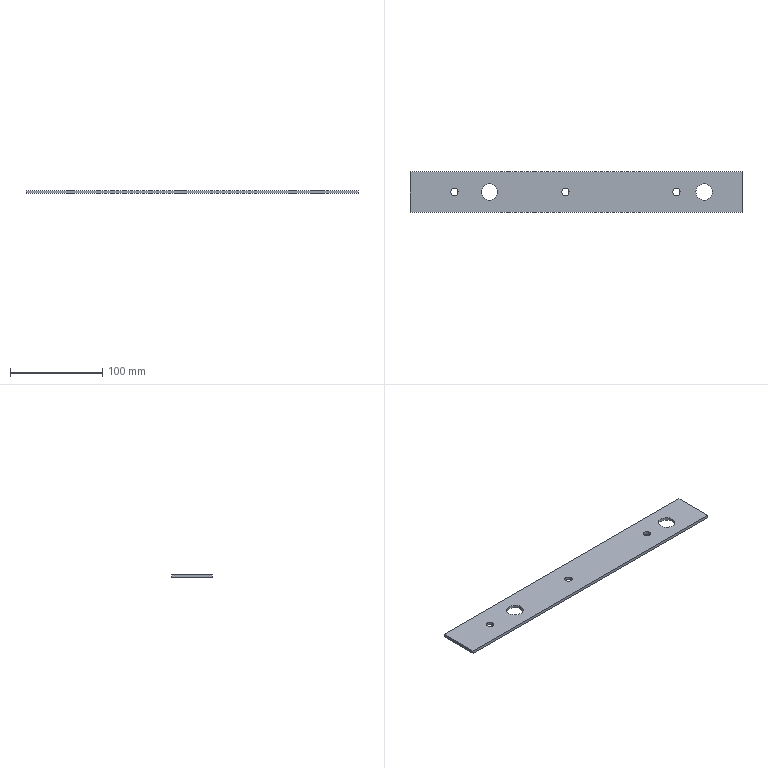Part | SolidWorks | features FlatPattern 1, SMBaseFlange 1, SheetMetal 1 | 1 solid | 16 faces | box 359 x 44 x 3.2 mm | volume 48436 mm3 | cylinder 10 | plane 6 | commonest cylinder face diameters 8 x6 18 x4
STEP:
#1=CARTESIAN_POINT('',(44.,-22.,-3.2));
#2=VERTEX_POINT('',#1);
#3=CARTESIAN_POINT('',(52.,-22.,-3.2));
#4=VERTEX_POINT('',#3);
#5=CARTESIAN_POINT('',(48.,-22.,-3.2));
#6=DIRECTION('',(0.,0.,1.));
#7=DIRECTION('',(1.,0.,0.));
#8=AXIS2_PLACEMENT_3D('',#5,#6,#7);
#9=CIRCLE('',#8,4.);
#10=EDGE_CURVE('',#2,#4,#9,.T.);
#11=ORIENTED_EDGE('',*,*,#10,.F.);
#12=CARTESIAN_POINT('',(44.,-22.,0.));
#13=VERTEX_POINT('',#12);
#14=CARTESIAN_POINT('',(44.,-22.,-3.2));
#15=DIRECTION('',(0.,0.,1.));
#16=VECTOR('',#15,1000.);
#17=LINE('',#14,#16);
#18=EDGE_CURVE('',#2,#13,#17,.T.);
#19=ORIENTED_EDGE('',*,*,#18,.T.);
#20=CARTESIAN_POINT('',(52.,-22.,0.));
#21=VERTEX_POINT('',#20);
#22=CARTESIAN_POINT('',(48.,-22.,0.));
#23=DIRECTION('',(0.,0.,1.));
#24=DIRECTION('',(1.,0.,0.));
#25=AXIS2_PLACEMENT_3D('',#22,#23,#24);
#26=CIRCLE('',#25,4.);
#27=EDGE_CURVE('',#13,#21,#26,.T.);
#28=ORIENTED_EDGE('',*,*,#27,.T.);
#29=CARTESIAN_POINT('',(52.,-22.,-3.2));
#30=DIRECTION('',(0.,0.,1.));
#31=VECTOR('',#30,1000.);
#32=LINE('',#29,#31);
#33=EDGE_CURVE('',#4,#21,#32,.T.);
#34=ORIENTED_EDGE('',*,*,#33,.F.);
#35=EDGE_LOOP('',(#11,#19,#28,#34));
#36=FACE_OUTER_BOUND('',#35,.T.);
#37=CARTESIAN_POINT('',(48.,-22.,-3.2));
#38=DIRECTION('',(0.,0.,1.));
#39=DIRECTION('',(1.,0.,0.));
#40=AXIS2_PLACEMENT_3D('',#37,#38,#39);
#41=CYLINDRICAL_SURFACE('',#40,4.);
#42=ADVANCED_FACE('',(#36),#41,.F.);
#43=CARTESIAN_POINT('',(164.,-22.,-3.2));
#44=VERTEX_POINT('',#43);
#45=CARTESIAN_POINT('',(172.,-22.,-3.2));
#46=VERTEX_POINT('',#45);
#47=CARTESIAN_POINT('',(168.,-22.,-3.2));
#48=DIRECTION('',(0.,0.,1.));
#49=DIRECTION('',(1.,0.,0.));
#50=AXIS2_PLACEMENT_3D('',#47,#48,#49);
#51=CIRCLE('',#50,4.);
#52=EDGE_CURVE('',#44,#46,#51,.T.);
#53=ORIENTED_EDGE('',*,*,#52,.F.);
#54=CARTESIAN_POINT('',(164.,-22.,0.));
#55=VERTEX_POINT('',#54);
#56=CARTESIAN_POINT('',(164.,-22.,-3.2));
#57=DIRECTION('',(0.,0.,1.));
#58=VECTOR('',#57,1000.);
#59=LINE('',#56,#58);
#60=EDGE_CURVE('',#44,#55,#59,.T.);
#61=ORIENTED_EDGE('',*,*,#60,.T.);
#62=CARTESIAN_POINT('',(172.,-22.,0.));
#63=VERTEX_POINT('',#62);
#64=CARTESIAN_POINT('',(168.,-22.,0.));
#65=DIRECTION('',(0.,0.,1.));
#66=DIRECTION('',(1.,0.,0.));
#67=AXIS2_PLACEMENT_3D('',#64,#65,#66);
#68=CIRCLE('',#67,4.);
#69=EDGE_CURVE('',#55,#63,#68,.T.);
#70=ORIENTED_EDGE('',*,*,#69,.T.);
#71=CARTESIAN_POINT('',(172.,-22.,-3.2));
#72=DIRECTION('',(0.,0.,1.));
#73=VECTOR('',#72,1000.);
#74=LINE('',#71,#73);
#75=EDGE_CURVE('',#46,#63,#74,.T.);
#76=ORIENTED_EDGE('',*,*,#75,.F.);
#77=EDGE_LOOP('',(#53,#61,#70,#76));
#78=FACE_OUTER_BOUND('',#77,.T.);
#79=CARTESIAN_POINT('',(168.,-22.,-3.2));
#80=DIRECTION('',(0.,0.,1.));
#81=DIRECTION('',(1.,0.,0.));
#82=AXIS2_PLACEMENT_3D('',#79,#80,#81);
#83=CYLINDRICAL_SURFACE('',#82,4.);
#84=ADVANCED_FACE('',(#78),#83,.F.);
#85=CARTESIAN_POINT('',(284.,-22.,-3.2));
#86=VERTEX_POINT('',#85);
#87=CARTESIAN_POINT('',(292.,-22.,-3.2));
#88=VERTEX_POINT('',#87);
#89=CARTESIAN_POINT('',(288.,-22.,-3.2));
#90=DIRECTION('',(0.,0.,1.));
#91=DIRECTION('',(1.,0.,0.));
#92=AXIS2_PLACEMENT_3D('',#89,#90,#91);
#93=CIRCLE('',#92,4.);
#94=EDGE_CURVE('',#86,#88,#93,.T.);
#95=ORIENTED_EDGE('',*,*,#94,.F.);
#96=CARTESIAN_POINT('',(284.,-22.,0.));
#97=VERTEX_POINT('',#96);
#98=CARTESIAN_POINT('',(284.,-22.,-3.2));
#99=DIRECTION('',(0.,0.,1.));
#100=VECTOR('',#99,1000.);
#101=LINE('',#98,#100);
#102=EDGE_CURVE('',#86,#97,#101,.T.);
#103=ORIENTED_EDGE('',*,*,#102,.T.);
#104=CARTESIAN_POINT('',(292.,-22.,0.));
#105=VERTEX_POINT('',#104);
#106=CARTESIAN_POINT('',(288.,-22.,0.));
#107=DIRECTION('',(0.,0.,1.));
#108=DIRECTION('',(1.,0.,0.));
#109=AXIS2_PLACEMENT_3D('',#106,#107,#108);
#110=CIRCLE('',#109,4.);
#111=EDGE_CURVE('',#97,#105,#110,.T.);
#112=ORIENTED_EDGE('',*,*,#111,.T.);
#113=CARTESIAN_POINT('',(292.,-22.,-3.2));
#114=DIRECTION('',(0.,0.,1.));
#115=VECTOR('',#114,1000.);
#116=LINE('',#113,#115);
#117=EDGE_CURVE('',#88,#105,#116,.T.);
#118=ORIENTED_EDGE('',*,*,#117,.F.);
#119=EDGE_LOOP('',(#95,#103,#112,#118));
#120=FACE_OUTER_BOUND('',#119,.T.);
#121=CARTESIAN_POINT('',(288.,-22.,-3.2));
#122=DIRECTION('',(0.,0.,1.));
#123=DIRECTION('',(1.,0.,0.));
#124=AXIS2_PLACEMENT_3D('',#121,#122,#123);
#125=CYLINDRICAL_SURFACE('',#124,4.);
#126=ADVANCED_FACE('',(#120),#125,.F.);
#127=CARTESIAN_POINT('',(77.,-22.,-3.2));
#128=VERTEX_POINT('',#127);
#129=CARTESIAN_POINT('',(95.,-22.,-3.2));
#130=VERTEX_POINT('',#129);
#131=CARTESIAN_POINT('',(86.,-22.,-3.2));
#132=DIRECTION('',(0.,0.,1.));
#133=DIRECTION('',(1.,0.,0.));
#134=AXIS2_PLACEMENT_3D('',#131,#132,#133);
#135=CIRCLE('',#134,9.);
#136=EDGE_CURVE('',#128,#130,#135,.T.);
#137=ORIENTED_EDGE('',*,*,#136,.F.);
#138=CARTESIAN_POINT('',(77.,-22.,0.));
#139=VERTEX_POINT('',#138);
#140=CARTESIAN_POINT('',(77.,-22.,-3.2));
#141=DIRECTION('',(0.,0.,1.));
#142=VECTOR('',#141,1000.);
#143=LINE('',#140,#142);
#144=EDGE_CURVE('',#128,#139,#143,.T.);
#145=ORIENTED_EDGE('',*,*,#144,.T.);
#146=CARTESIAN_POINT('',(95.,-22.,0.));
#147=VERTEX_POINT('',#146);
#148=CARTESIAN_POINT('',(86.,-22.,0.));
#149=DIRECTION('',(0.,0.,1.));
#150=DIRECTION('',(1.,0.,0.));
#151=AXIS2_PLACEMENT_3D('',#148,#149,#150);
#152=CIRCLE('',#151,9.);
#153=EDGE_CURVE('',#139,#147,#152,.T.);
#154=ORIENTED_EDGE('',*,*,#153,.T.);
#155=CARTESIAN_POINT('',(95.,-22.,-3.2));
#156=DIRECTION('',(0.,0.,1.));
#157=VECTOR('',#156,1000.);
#158=LINE('',#155,#157);
#159=EDGE_CURVE('',#130,#147,#158,.T.);
#160=ORIENTED_EDGE('',*,*,#159,.F.);
#161=EDGE_LOOP('',(#137,#145,#154,#160));
#162=FACE_OUTER_BOUND('',#161,.T.);
#163=CARTESIAN_POINT('',(86.,-22.,-3.2));
#164=DIRECTION('',(0.,0.,1.));
#165=DIRECTION('',(1.,0.,0.));
#166=AXIS2_PLACEMENT_3D('',#163,#164,#165);
#167=CYLINDRICAL_SURFACE('',#166,9.);
#168=ADVANCED_FACE('',(#162),#167,.F.);
#169=CARTESIAN_POINT('',(309.,-22.,-3.2));
#170=VERTEX_POINT('',#169);
#171=CARTESIAN_POINT('',(327.,-22.,-3.2));
#172=VERTEX_POINT('',#171);
#173=CARTESIAN_POINT('',(318.,-22.,-3.2));
#174=DIRECTION('',(0.,0.,1.));
#175=DIRECTION('',(1.,0.,0.));
#176=AXIS2_PLACEMENT_3D('',#173,#174,#175);
#177=CIRCLE('',#176,9.);
#178=EDGE_CURVE('',#170,#172,#177,.T.);
#179=ORIENTED_EDGE('',*,*,#178,.F.);
#180=CARTESIAN_POINT('',(309.,-22.,0.));
#181=VERTEX_POINT('',#180);
#182=CARTESIAN_POINT('',(309.,-22.,-3.2));
#183=DIRECTION('',(0.,0.,1.));
#184=VECTOR('',#183,1000.);
#185=LINE('',#182,#184);
#186=EDGE_CURVE('',#170,#181,#185,.T.);
#187=ORIENTED_EDGE('',*,*,#186,.T.);
#188=CARTESIAN_POINT('',(327.,-22.,0.));
#189=VERTEX_POINT('',#188);
#190=CARTESIAN_POINT('',(318.,-22.,0.));
#191=DIRECTION('',(0.,0.,1.));
#192=DIRECTION('',(1.,0.,0.));
#193=AXIS2_PLACEMENT_3D('',#190,#191,#192);
#194=CIRCLE('',#193,9.);
#195=EDGE_CURVE('',#181,#189,#194,.T.);
#196=ORIENTED_EDGE('',*,*,#195,.T.);
#197=CARTESIAN_POINT('',(327.,-22.,-3.2));
#198=DIRECTION('',(0.,0.,1.));
#199=VECTOR('',#198,1000.);
#200=LINE('',#197,#199);
#201=EDGE_CURVE('',#172,#189,#200,.T.);
#202=ORIENTED_EDGE('',*,*,#201,.F.);
#203=EDGE_LOOP('',(#179,#187,#196,#202));
#204=FACE_OUTER_BOUND('',#203,.T.);
#205=CARTESIAN_POINT('',(318.,-22.,-3.2));
#206=DIRECTION('',(0.,0.,1.));
#207=DIRECTION('',(1.,0.,0.));
#208=AXIS2_PLACEMENT_3D('',#205,#206,#207);
#209=CYLINDRICAL_SURFACE('',#208,9.);
#210=ADVANCED_FACE('',(#204),#209,.F.);
#211=CARTESIAN_POINT('',(0.,0.,0.));
#212=VERTEX_POINT('',#211);
#213=CARTESIAN_POINT('',(0.,-44.,0.));
#214=VERTEX_POINT('',#213);
#215=CARTESIAN_POINT('',(0.,0.,0.));
#216=DIRECTION('',(0.,-1.,0.));
#217=VECTOR('',#216,1000.);
#218=LINE('',#215,#217);
#219=EDGE_CURVE('',#212,#214,#218,.T.);
#220=ORIENTED_EDGE('',*,*,#219,.F.);
#221=CARTESIAN_POINT('',(0.,0.,-3.2));
#222=VERTEX_POINT('',#221);
#223=CARTESIAN_POINT('',(0.,0.,-3.2));
#224=DIRECTION('',(0.,0.,1.));
#225=VECTOR('',#224,1000.);
#226=LINE('',#223,#225);
#227=EDGE_CURVE('',#222,#212,#226,.T.);
#228=ORIENTED_EDGE('',*,*,#227,.F.);
#229=CARTESIAN_POINT('',(0.,-44.,-3.2));
#230=VERTEX_POINT('',#229);
#231=CARTESIAN_POINT('',(0.,0.,-3.2));
#232=DIRECTION('',(0.,-1.,0.));
#233=VECTOR('',#232,1000.);
#234=LINE('',#231,#233);
#235=EDGE_CURVE('',#222,#230,#234,.T.);
#236=ORIENTED_EDGE('',*,*,#235,.T.);
#237=CARTESIAN_POINT('',(0.,-44.,-3.2));
#238=DIRECTION('',(0.,0.,1.));
#239=VECTOR('',#238,1000.);
#240=LINE('',#237,#239);
#241=EDGE_CURVE('',#230,#214,#240,.T.);
#242=ORIENTED_EDGE('',*,*,#241,.T.);
#243=EDGE_LOOP('',(#220,#228,#236,#242));
#244=FACE_OUTER_BOUND('',#243,.T.);
#245=CARTESIAN_POINT('',(0.,0.,-3.2));
#246=DIRECTION('',(-1.,0.,0.));
#247=DIRECTION('',(0.,0.,1.));
#248=AXIS2_PLACEMENT_3D('',#245,#246,#247);
#249=PLANE('',#248);
#250=ADVANCED_FACE('',(#244),#249,.T.);
#251=CARTESIAN_POINT('',(359.,0.,0.));
#252=VERTEX_POINT('',#251);
#253=CARTESIAN_POINT('',(0.,0.,0.));
#254=DIRECTION('',(-1.,0.,0.));
#255=VECTOR('',#254,1000.);
#256=LINE('',#253,#255);
#257=EDGE_CURVE('',#252,#212,#256,.T.);
#258=ORIENTED_EDGE('',*,*,#257,.F.);
#259=CARTESIAN_POINT('',(359.,0.,-3.2));
#260=VERTEX_POINT('',#259);
#261=CARTESIAN_POINT('',(359.,0.,-3.2));
#262=DIRECTION('',(0.,0.,1.));
#263=VECTOR('',#262,1000.);
#264=LINE('',#261,#263);
#265=EDGE_CURVE('',#260,#252,#264,.T.);
#266=ORIENTED_EDGE('',*,*,#265,.F.);
#267=CARTESIAN_POINT('',(0.,0.,-3.2));
#268=DIRECTION('',(-1.,0.,0.));
#269=VECTOR('',#268,1000.);
#270=LINE('',#267,#269);
#271=EDGE_CURVE('',#260,#222,#270,.T.);
#272=ORIENTED_EDGE('',*,*,#271,.T.);
#273=ORIENTED_EDGE('',*,*,#227,.T.);
#274=EDGE_LOOP('',(#258,#266,#272,#273));
#275=FACE_OUTER_BOUND('',#274,.T.);
#276=CARTESIAN_POINT('',(0.,0.,-3.2));
#277=DIRECTION('',(0.,1.,0.));
#278=DIRECTION('',(0.,0.,1.));
#279=AXIS2_PLACEMENT_3D('',#276,#277,#278);
#280=PLANE('',#279);
#281=ADVANCED_FACE('',(#275),#280,.T.);
#282=CARTESIAN_POINT('',(359.,-44.,0.));
#283=VERTEX_POINT('',#282);
#284=CARTESIAN_POINT('',(359.,0.,0.));
#285=DIRECTION('',(0.,1.,0.));
#286=VECTOR('',#285,1000.);
#287=LINE('',#284,#286);
#288=EDGE_CURVE('',#283,#252,#287,.T.);
#289=ORIENTED_EDGE('',*,*,#288,.F.);
#290=CARTESIAN_POINT('',(359.,-44.,-3.2));
#291=VERTEX_POINT('',#290);
#292=CARTESIAN_POINT('',(359.,-44.,-3.2));
#293=DIRECTION('',(0.,0.,1.));
#294=VECTOR('',#293,1000.);
#295=LINE('',#292,#294);
#296=EDGE_CURVE('',#291,#283,#295,.T.);
#297=ORIENTED_EDGE('',*,*,#296,.F.);
#298=CARTESIAN_POINT('',(359.,0.,-3.2));
#299=DIRECTION('',(0.,1.,0.));
#300=VECTOR('',#299,1000.);
#301=LINE('',#298,#300);
#302=EDGE_CURVE('',#291,#260,#301,.T.);
#303=ORIENTED_EDGE('',*,*,#302,.T.);
#304=ORIENTED_EDGE('',*,*,#265,.T.);
#305=EDGE_LOOP('',(#289,#297,#303,#304));
#306=FACE_OUTER_BOUND('',#305,.T.);
#307=CARTESIAN_POINT('',(359.,0.,-3.2));
#308=DIRECTION('',(1.,0.,0.));
#309=DIRECTION('',(0.,0.,-1.));
#310=AXIS2_PLACEMENT_3D('',#307,#308,#309);
#311=PLANE('',#310);
#312=ADVANCED_FACE('',(#306),#311,.T.);
#313=CARTESIAN_POINT('',(0.,-44.,0.));
#314=DIRECTION('',(1.,0.,0.));
#315=VECTOR('',#314,1000.);
#316=LINE('',#313,#315);
#317=EDGE_CURVE('',#214,#283,#316,.T.);
#318=ORIENTED_EDGE('',*,*,#317,.F.);
#319=ORIENTED_EDGE('',*,*,#241,.F.);
#320=CARTESIAN_POINT('',(0.,-44.,-3.2));
#321=DIRECTION('',(1.,0.,0.));
#322=VECTOR('',#321,1000.);
#323=LINE('',#320,#322);
#324=EDGE_CURVE('',#230,#291,#323,.T.);
#325=ORIENTED_EDGE('',*,*,#324,.T.);
#326=ORIENTED_EDGE('',*,*,#296,.T.);
#327=EDGE_LOOP('',(#318,#319,#325,#326));
#328=FACE_OUTER_BOUND('',#327,.T.);
#329=CARTESIAN_POINT('',(0.,-44.,-3.2));
#330=DIRECTION('',(0.,-1.,0.));
#331=DIRECTION('',(0.,0.,-1.));
#332=AXIS2_PLACEMENT_3D('',#329,#330,#331);
#333=PLANE('',#332);
#334=ADVANCED_FACE('',(#328),#333,.T.);
#335=CARTESIAN_POINT('',(48.,-22.,-3.2));
#336=DIRECTION('',(0.,0.,1.));
#337=DIRECTION('',(1.,0.,0.));
#338=AXIS2_PLACEMENT_3D('',#335,#336,#337);
#339=CIRCLE('',#338,4.);
#340=EDGE_CURVE('',#4,#2,#339,.T.);
#341=ORIENTED_EDGE('',*,*,#340,.T.);
#342=ORIENTED_EDGE('',*,*,#10,.T.);
#343=EDGE_LOOP('',(#341,#342));
#344=FACE_BOUND('',#343,.T.);
#345=CARTESIAN_POINT('',(168.,-22.,-3.2));
#346=DIRECTION('',(0.,0.,1.));
#347=DIRECTION('',(1.,0.,0.));
#348=AXIS2_PLACEMENT_3D('',#345,#346,#347);
#349=CIRCLE('',#348,4.);
#350=EDGE_CURVE('',#46,#44,#349,.T.);
#351=ORIENTED_EDGE('',*,*,#350,.T.);
#352=ORIENTED_EDGE('',*,*,#52,.T.);
#353=EDGE_LOOP('',(#351,#352));
#354=FACE_BOUND('',#353,.T.);
#355=CARTESIAN_POINT('',(288.,-22.,-3.2));
#356=DIRECTION('',(0.,0.,1.));
#357=DIRECTION('',(1.,0.,0.));
#358=AXIS2_PLACEMENT_3D('',#355,#356,#357);
#359=CIRCLE('',#358,4.);
#360=EDGE_CURVE('',#88,#86,#359,.T.);
#361=ORIENTED_EDGE('',*,*,#360,.T.);
#362=ORIENTED_EDGE('',*,*,#94,.T.);
#363=EDGE_LOOP('',(#361,#362));
#364=FACE_BOUND('',#363,.T.);
#365=CARTESIAN_POINT('',(86.,-22.,-3.2));
#366=DIRECTION('',(0.,0.,1.));
#367=DIRECTION('',(1.,0.,0.));
#368=AXIS2_PLACEMENT_3D('',#365,#366,#367);
#369=CIRCLE('',#368,9.);
#370=EDGE_CURVE('',#130,#128,#369,.T.);
#371=ORIENTED_EDGE('',*,*,#370,.T.);
#372=ORIENTED_EDGE('',*,*,#136,.T.);
#373=EDGE_LOOP('',(#371,#372));
#374=FACE_BOUND('',#373,.T.);
#375=CARTESIAN_POINT('',(318.,-22.,-3.2));
#376=DIRECTION('',(0.,0.,1.));
#377=DIRECTION('',(1.,0.,0.));
#378=AXIS2_PLACEMENT_3D('',#375,#376,#377);
#379=CIRCLE('',#378,9.);
#380=EDGE_CURVE('',#172,#170,#379,.T.);
#381=ORIENTED_EDGE('',*,*,#380,.T.);
#382=ORIENTED_EDGE('',*,*,#178,.T.);
#383=EDGE_LOOP('',(#381,#382));
#384=FACE_BOUND('',#383,.T.);
#385=ORIENTED_EDGE('',*,*,#235,.F.);
#386=ORIENTED_EDGE('',*,*,#271,.F.);
#387=ORIENTED_EDGE('',*,*,#302,.F.);
#388=ORIENTED_EDGE('',*,*,#324,.F.);
#389=EDGE_LOOP('',(#385,#386,#387,#388));
#390=FACE_OUTER_BOUND('',#389,.T.);
#391=CARTESIAN_POINT('',(0.,0.,-3.2));
#392=DIRECTION('',(0.,0.,1.));
#393=DIRECTION('',(1.,0.,0.));
#394=AXIS2_PLACEMENT_3D('',#391,#392,#393);
#395=PLANE('',#394);
#396=ADVANCED_FACE('',(#344,#354,#364,#374,#384,#390),#395,.F.);
#397=CARTESIAN_POINT('',(48.,-22.,0.));
#398=DIRECTION('',(0.,0.,1.));
#399=DIRECTION('',(1.,0.,0.));
#400=AXIS2_PLACEMENT_3D('',#397,#398,#399);
#401=CIRCLE('',#400,4.);
#402=EDGE_CURVE('',#21,#13,#401,.T.);
#403=ORIENTED_EDGE('',*,*,#402,.F.);
#404=ORIENTED_EDGE('',*,*,#27,.F.);
#405=EDGE_LOOP('',(#403,#404));
#406=FACE_BOUND('',#405,.T.);
#407=CARTESIAN_POINT('',(168.,-22.,0.));
#408=DIRECTION('',(0.,0.,1.));
#409=DIRECTION('',(1.,0.,0.));
#410=AXIS2_PLACEMENT_3D('',#407,#408,#409);
#411=CIRCLE('',#410,4.);
#412=EDGE_CURVE('',#63,#55,#411,.T.);
#413=ORIENTED_EDGE('',*,*,#412,.F.);
#414=ORIENTED_EDGE('',*,*,#69,.F.);
#415=EDGE_LOOP('',(#413,#414));
#416=FACE_BOUND('',#415,.T.);
#417=CARTESIAN_POINT('',(288.,-22.,0.));
#418=DIRECTION('',(0.,0.,1.));
#419=DIRECTION('',(1.,0.,0.));
#420=AXIS2_PLACEMENT_3D('',#417,#418,#419);
#421=CIRCLE('',#420,4.);
#422=EDGE_CURVE('',#105,#97,#421,.T.);
#423=ORIENTED_EDGE('',*,*,#422,.F.);
#424=ORIENTED_EDGE('',*,*,#111,.F.);
#425=EDGE_LOOP('',(#423,#424));
#426=FACE_BOUND('',#425,.T.);
#427=CARTESIAN_POINT('',(86.,-22.,0.));
#428=DIRECTION('',(0.,0.,1.));
#429=DIRECTION('',(1.,0.,0.));
#430=AXIS2_PLACEMENT_3D('',#427,#428,#429);
#431=CIRCLE('',#430,9.);
#432=EDGE_CURVE('',#147,#139,#431,.T.);
#433=ORIENTED_EDGE('',*,*,#432,.F.);
#434=ORIENTED_EDGE('',*,*,#153,.F.);
#435=EDGE_LOOP('',(#433,#434));
#436=FACE_BOUND('',#435,.T.);
#437=CARTESIAN_POINT('',(318.,-22.,0.));
#438=DIRECTION('',(0.,0.,1.));
#439=DIRECTION('',(1.,0.,0.));
#440=AXIS2_PLACEMENT_3D('',#437,#438,#439);
#441=CIRCLE('',#440,9.);
#442=EDGE_CURVE('',#189,#181,#441,.T.);
#443=ORIENTED_EDGE('',*,*,#442,.F.);
#444=ORIENTED_EDGE('',*,*,#195,.F.);
#445=EDGE_LOOP('',(#443,#444));
#446=FACE_BOUND('',#445,.T.);
#447=ORIENTED_EDGE('',*,*,#219,.T.);
#448=ORIENTED_EDGE('',*,*,#317,.T.);
#449=ORIENTED_EDGE('',*,*,#288,.T.);
#450=ORIENTED_EDGE('',*,*,#257,.T.);
#451=EDGE_LOOP('',(#447,#448,#449,#450));
#452=FACE_OUTER_BOUND('',#451,.T.);
#453=CARTESIAN_POINT('',(0.,0.,0.));
#454=DIRECTION('',(0.,0.,1.));
#455=DIRECTION('',(1.,0.,0.));
#456=AXIS2_PLACEMENT_3D('',#453,#454,#455);
#457=PLANE('',#456);
#458=ADVANCED_FACE('',(#406,#416,#426,#436,#446,#452),#457,.T.);
#459=ORIENTED_EDGE('',*,*,#186,.F.);
#460=ORIENTED_EDGE('',*,*,#380,.F.);
#461=ORIENTED_EDGE('',*,*,#201,.T.);
#462=ORIENTED_EDGE('',*,*,#442,.T.);
#463=EDGE_LOOP('',(#459,#460,#461,#462));
#464=FACE_OUTER_BOUND('',#463,.T.);
#465=CARTESIAN_POINT('',(318.,-22.,-3.2));
#466=DIRECTION('',(0.,0.,1.));
#467=DIRECTION('',(1.,0.,0.));
#468=AXIS2_PLACEMENT_3D('',#465,#466,#467);
#469=CYLINDRICAL_SURFACE('',#468,9.);
#470=ADVANCED_FACE('',(#464),#469,.F.);
#471=ORIENTED_EDGE('',*,*,#144,.F.);
#472=ORIENTED_EDGE('',*,*,#370,.F.);
#473=ORIENTED_EDGE('',*,*,#159,.T.);
#474=ORIENTED_EDGE('',*,*,#432,.T.);
#475=EDGE_LOOP('',(#471,#472,#473,#474));
#476=FACE_OUTER_BOUND('',#475,.T.);
#477=CARTESIAN_POINT('',(86.,-22.,-3.2));
#478=DIRECTION('',(0.,0.,1.));
#479=DIRECTION('',(1.,0.,0.));
#480=AXIS2_PLACEMENT_3D('',#477,#478,#479);
#481=CYLINDRICAL_SURFACE('',#480,9.);
#482=ADVANCED_FACE('',(#476),#481,.F.);
#483=ORIENTED_EDGE('',*,*,#102,.F.);
#484=ORIENTED_EDGE('',*,*,#360,.F.);
#485=ORIENTED_EDGE('',*,*,#117,.T.);
#486=ORIENTED_EDGE('',*,*,#422,.T.);
#487=EDGE_LOOP('',(#483,#484,#485,#486));
#488=FACE_OUTER_BOUND('',#487,.T.);
#489=CARTESIAN_POINT('',(288.,-22.,-3.2));
#490=DIRECTION('',(0.,0.,1.));
#491=DIRECTION('',(1.,0.,0.));
#492=AXIS2_PLACEMENT_3D('',#489,#490,#491);
#493=CYLINDRICAL_SURFACE('',#492,4.);
#494=ADVANCED_FACE('',(#488),#493,.F.);
#495=ORIENTED_EDGE('',*,*,#60,.F.);
#496=ORIENTED_EDGE('',*,*,#350,.F.);
#497=ORIENTED_EDGE('',*,*,#75,.T.);
#498=ORIENTED_EDGE('',*,*,#412,.T.);
#499=EDGE_LOOP('',(#495,#496,#497,#498));
#500=FACE_OUTER_BOUND('',#499,.T.);
#501=CARTESIAN_POINT('',(168.,-22.,-3.2));
#502=DIRECTION('',(0.,0.,1.));
#503=DIRECTION('',(1.,0.,0.));
#504=AXIS2_PLACEMENT_3D('',#501,#502,#503);
#505=CYLINDRICAL_SURFACE('',#504,4.);
#506=ADVANCED_FACE('',(#500),#505,.F.);
#507=ORIENTED_EDGE('',*,*,#18,.F.);
#508=ORIENTED_EDGE('',*,*,#340,.F.);
#509=ORIENTED_EDGE('',*,*,#33,.T.);
#510=ORIENTED_EDGE('',*,*,#402,.T.);
#511=EDGE_LOOP('',(#507,#508,#509,#510));
#512=FACE_OUTER_BOUND('',#511,.T.);
#513=CARTESIAN_POINT('',(48.,-22.,-3.2));
#514=DIRECTION('',(0.,0.,1.));
#515=DIRECTION('',(1.,0.,0.));
#516=AXIS2_PLACEMENT_3D('',#513,#514,#515);
#517=CYLINDRICAL_SURFACE('',#516,4.);
#518=ADVANCED_FACE('',(#512),#517,.F.);
#519=CLOSED_SHELL('',(#42,#84,#126,#168,#210,#250,#281,#312,#334,#396,#458,#470,#482,#494,#506,#518));
#520=MANIFOLD_SOLID_BREP('',#519);
#521=CARTESIAN_POINT('',(0.,0.,0.));
#522=DIRECTION('',(0.,0.,1.));
#523=DIRECTION('',(1.,0.,0.));
#524=AXIS2_PLACEMENT_3D('',#521,#522,#523);
#525=(LENGTH_UNIT()NAMED_UNIT(*)SI_UNIT(.MILLI.,.METRE.));
#526=UNCERTAINTY_MEASURE_WITH_UNIT(LENGTH_MEASURE(0.00001),#525,'','');
#527=(NAMED_UNIT(*)PLANE_ANGLE_UNIT()SI_UNIT($,.RADIAN.));
#528=(NAMED_UNIT(*)SI_UNIT($,.STERADIAN.)SOLID_ANGLE_UNIT());
#529=(GEOMETRIC_REPRESENTATION_CONTEXT(3)GLOBAL_UNCERTAINTY_ASSIGNED_CONTEXT((#526))GLOBAL_UNIT_ASSIGNED_CONTEXT((#525,#527,#528))REPRESENTATION_CONTEXT('',''));
#530=ADVANCED_BREP_SHAPE_REPRESENTATION('',(#520,#524),#529);